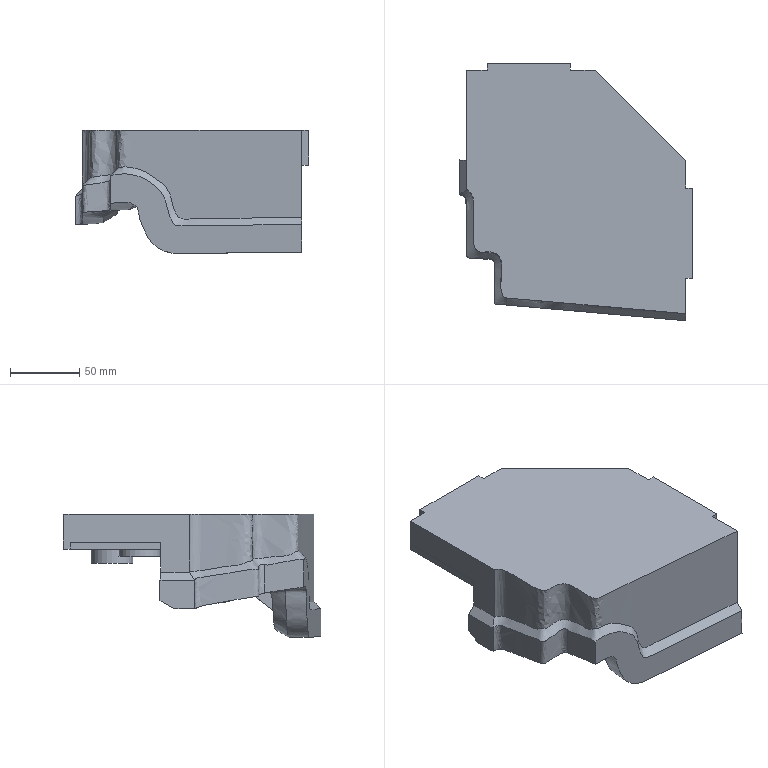Part | NX | features solid 2 | 1 solid | 38 faces | box 168 x 185.503 x 88.687 mm | volume 912814 mm3 | plane 25 | spline 8 | cylinder 5 | commonest cylinder face diameters 30 x5